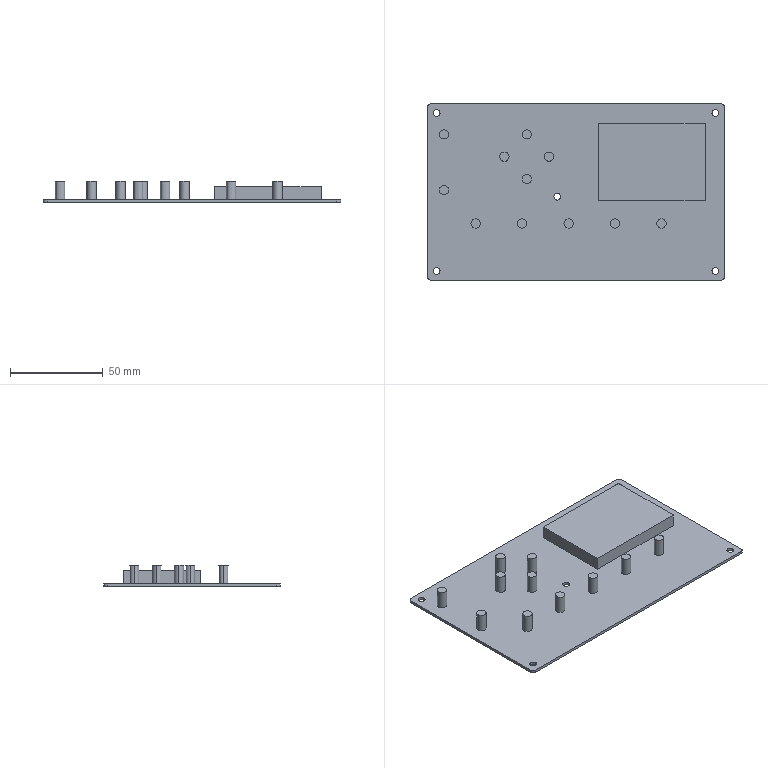Part | SolidWorks | features BaseBody 1 | 1 solid | 58 faces | box 160 x 95 x 11.5 mm | volume 41578 mm3 | cylinder 36 | plane 22 | commonest cylinder face diameters 5 x22 3.7 x10 4 x4